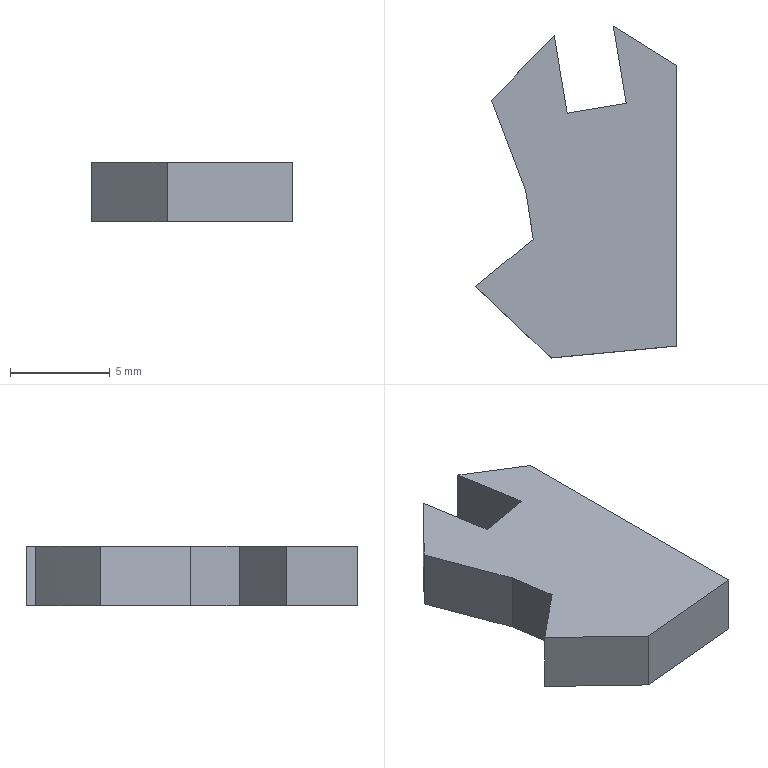Part | SolidWorks | features BaseBody 1 | 1 solid | 13 faces | box 10.052 x 16.622 x 3 mm | volume 347.373 mm3 | spline 7 | plane 6
STEP:
#1=CARTESIAN_POINT('',(-6.421,0.002241,-1.5));
#2=VERTEX_POINT('',#1);
#3=CARTESIAN_POINT('',(-0.1475,0.5984,-1.5));
#4=VERTEX_POINT('',#3);
#5=CARTESIAN_POINT('',(-6.421,0.002241,-1.5));
#6=CARTESIAN_POINT('',(-4.332,0.1996,-1.5));
#7=CARTESIAN_POINT('',(-0.1475,0.5984,-1.5));
#8=B_SPLINE_CURVE_WITH_KNOTS('',2,(#5,#6,#7),.UNSPECIFIED.,.F.,.F.,(3,3),(0.,0.05556),.UNSPECIFIED.);
#9=EDGE_CURVE('',#2,#4,#8,.T.);
#10=ORIENTED_EDGE('',*,*,#9,.F.);
#11=CARTESIAN_POINT('',(-10.2,3.587,-1.5));
#12=VERTEX_POINT('',#11);
#13=CARTESIAN_POINT('',(-10.2,3.587,-1.5));
#14=CARTESIAN_POINT('',(-8.939,2.393,-1.5));
#15=CARTESIAN_POINT('',(-7.681,1.198,-1.5));
#16=CARTESIAN_POINT('',(-6.421,0.002241,-1.5));
#17=B_SPLINE_CURVE_WITH_KNOTS('',3,(#13,#14,#15,#16),.UNSPECIFIED.,.F.,.F.,(4,4),(0.05556,0.1111),.UNSPECIFIED.);
#18=EDGE_CURVE('',#12,#2,#17,.T.);
#19=ORIENTED_EDGE('',*,*,#18,.F.);
#20=CARTESIAN_POINT('',(-7.315,5.947,-1.5));
#21=VERTEX_POINT('',#20);
#22=CARTESIAN_POINT('',(-7.315,5.947,-1.5));
#23=CARTESIAN_POINT('',(-8.275,5.16,-1.5));
#24=CARTESIAN_POINT('',(-9.238,4.374,-1.5));
#25=CARTESIAN_POINT('',(-10.2,3.587,-1.5));
#26=B_SPLINE_CURVE_WITH_KNOTS('',3,(#22,#23,#24,#25),.UNSPECIFIED.,.F.,.F.,(4,4),(0.1111,0.1667),.UNSPECIFIED.);
#27=EDGE_CURVE('',#21,#12,#26,.T.);
#28=ORIENTED_EDGE('',*,*,#27,.F.);
#29=CARTESIAN_POINT('',(-7.695,8.398,-1.5));
#30=VERTEX_POINT('',#29);
#31=CARTESIAN_POINT('',(-7.695,8.398,-1.5));
#32=CARTESIAN_POINT('',(-7.57,7.58,-1.5));
#33=CARTESIAN_POINT('',(-7.442,6.765,-1.5));
#34=CARTESIAN_POINT('',(-7.315,5.947,-1.5));
#35=B_SPLINE_CURVE_WITH_KNOTS('',3,(#31,#32,#33,#34),.UNSPECIFIED.,.F.,.F.,(4,4),(0.1667,0.2222),.UNSPECIFIED.);
#36=EDGE_CURVE('',#30,#21,#35,.T.);
#37=ORIENTED_EDGE('',*,*,#36,.F.);
#38=CARTESIAN_POINT('',(-9.403,12.915,-1.5));
#39=VERTEX_POINT('',#38);
#40=CARTESIAN_POINT('',(-9.403,12.915,-1.5));
#41=CARTESIAN_POINT('',(-8.834,11.41,-1.5));
#42=CARTESIAN_POINT('',(-8.265,9.904,-1.5));
#43=CARTESIAN_POINT('',(-7.695,8.398,-1.5));
#44=B_SPLINE_CURVE_WITH_KNOTS('',3,(#40,#41,#42,#43),.UNSPECIFIED.,.F.,.F.,(4,4),(0.2222,0.2778),.UNSPECIFIED.);
#45=EDGE_CURVE('',#39,#30,#44,.T.);
#46=ORIENTED_EDGE('',*,*,#45,.F.);
#47=CARTESIAN_POINT('',(-6.263,16.129,-1.5));
#48=VERTEX_POINT('',#47);
#49=CARTESIAN_POINT('',(-6.263,16.129,-1.5));
#50=CARTESIAN_POINT('',(-8.357,13.987,-1.5));
#51=CARTESIAN_POINT('',(-9.403,12.915,-1.5));
#52=B_SPLINE_CURVE_WITH_KNOTS('',2,(#49,#50,#51),.UNSPECIFIED.,.F.,.F.,(3,3),(0.2778,0.3333),.UNSPECIFIED.);
#53=EDGE_CURVE('',#48,#39,#52,.T.);
#54=ORIENTED_EDGE('',*,*,#53,.F.);
#55=CARTESIAN_POINT('',(-5.612,12.258,-1.5));
#56=VERTEX_POINT('',#55);
#57=CARTESIAN_POINT('',(-5.612,12.258,-1.5));
#58=DIRECTION('',(-0.1659,0.9861,0.));
#59=VECTOR('',#58,1000.);
#60=LINE('',#57,#59);
#61=EDGE_CURVE('',#56,#48,#60,.T.);
#62=ORIENTED_EDGE('',*,*,#61,.F.);
#63=CARTESIAN_POINT('',(-2.654,12.756,-1.5));
#64=VERTEX_POINT('',#63);
#65=CARTESIAN_POINT('',(-2.654,12.756,-1.5));
#66=DIRECTION('',(-0.9861,-0.1659,0.));
#67=VECTOR('',#66,1000.);
#68=LINE('',#65,#67);
#69=EDGE_CURVE('',#64,#56,#68,.T.);
#70=ORIENTED_EDGE('',*,*,#69,.F.);
#71=CARTESIAN_POINT('',(-3.305,16.624,-1.5));
#72=VERTEX_POINT('',#71);
#73=CARTESIAN_POINT('',(-2.654,12.756,-1.5));
#74=DIRECTION('',(0.1659,-0.9861,0.));
#75=VECTOR('',#74,1000.);
#76=LINE('',#73,#75);
#77=EDGE_CURVE('',#72,#64,#76,.T.);
#78=ORIENTED_EDGE('',*,*,#77,.F.);
#79=CARTESIAN_POINT('',(-0.1475,14.641,-1.5));
#80=VERTEX_POINT('',#79);
#81=CARTESIAN_POINT('',(-0.1475,14.641,-1.5));
#82=CARTESIAN_POINT('',(-1.178,15.289,-1.5));
#83=CARTESIAN_POINT('',(-3.21,16.565,-1.5));
#84=CARTESIAN_POINT('',(-3.305,16.624,-1.5));
#85=B_SPLINE_CURVE_WITH_KNOTS('',3,(#81,#82,#83,#84),.UNSPECIFIED.,.F.,.F.,(4,4),(0.8346,0.8889),.UNSPECIFIED.);
#86=EDGE_CURVE('',#80,#72,#85,.T.);
#87=ORIENTED_EDGE('',*,*,#86,.F.);
#88=CARTESIAN_POINT('',(-0.1475,14.641,-1.5));
#89=DIRECTION('',(0.,1.,0.));
#90=VECTOR('',#89,1000.);
#91=LINE('',#88,#90);
#92=EDGE_CURVE('',#4,#80,#91,.T.);
#93=ORIENTED_EDGE('',*,*,#92,.F.);
#94=EDGE_LOOP('',(#10,#19,#28,#37,#46,#54,#62,#70,#78,#87,#93));
#95=FACE_OUTER_BOUND('',#94,.T.);
#96=CARTESIAN_POINT('',(-3.808,0.25,-1.5));
#97=DIRECTION('',(0.,0.,1.));
#98=DIRECTION('',(1.,0.,0.));
#99=AXIS2_PLACEMENT_3D('',#96,#97,#98);
#100=PLANE('',#99);
#101=ADVANCED_FACE('',(#95),#100,.F.);
#102=CARTESIAN_POINT('',(-6.421,0.002241,1.5));
#103=VERTEX_POINT('',#102);
#104=CARTESIAN_POINT('',(-0.1475,0.5984,1.5));
#105=VERTEX_POINT('',#104);
#106=CARTESIAN_POINT('',(-6.421,0.002241,1.5));
#107=CARTESIAN_POINT('',(-4.332,0.1996,1.5));
#108=CARTESIAN_POINT('',(-0.1475,0.5984,1.5));
#109=B_SPLINE_CURVE_WITH_KNOTS('',2,(#106,#107,#108),.UNSPECIFIED.,.F.,.F.,(3,3),(0.,0.05556),.UNSPECIFIED.);
#110=EDGE_CURVE('',#103,#105,#109,.T.);
#111=ORIENTED_EDGE('',*,*,#110,.T.);
#112=CARTESIAN_POINT('',(-0.1475,14.641,1.5));
#113=VERTEX_POINT('',#112);
#114=CARTESIAN_POINT('',(-0.1475,14.641,1.5));
#115=DIRECTION('',(0.,1.,0.));
#116=VECTOR('',#115,1000.);
#117=LINE('',#114,#116);
#118=EDGE_CURVE('',#105,#113,#117,.T.);
#119=ORIENTED_EDGE('',*,*,#118,.T.);
#120=CARTESIAN_POINT('',(-3.305,16.624,1.5));
#121=VERTEX_POINT('',#120);
#122=CARTESIAN_POINT('',(-0.1475,14.641,1.5));
#123=CARTESIAN_POINT('',(-1.178,15.289,1.5));
#124=CARTESIAN_POINT('',(-3.21,16.565,1.5));
#125=CARTESIAN_POINT('',(-3.305,16.624,1.5));
#126=B_SPLINE_CURVE_WITH_KNOTS('',3,(#122,#123,#124,#125),.UNSPECIFIED.,.F.,.F.,(4,4),(0.8346,0.8889),.UNSPECIFIED.);
#127=EDGE_CURVE('',#113,#121,#126,.T.);
#128=ORIENTED_EDGE('',*,*,#127,.T.);
#129=CARTESIAN_POINT('',(-2.654,12.756,1.5));
#130=VERTEX_POINT('',#129);
#131=CARTESIAN_POINT('',(-2.654,12.756,1.5));
#132=DIRECTION('',(0.1659,-0.9861,0.));
#133=VECTOR('',#132,1000.);
#134=LINE('',#131,#133);
#135=EDGE_CURVE('',#121,#130,#134,.T.);
#136=ORIENTED_EDGE('',*,*,#135,.T.);
#137=CARTESIAN_POINT('',(-5.612,12.258,1.5));
#138=VERTEX_POINT('',#137);
#139=CARTESIAN_POINT('',(-2.654,12.756,1.5));
#140=DIRECTION('',(-0.9861,-0.1659,0.));
#141=VECTOR('',#140,1000.);
#142=LINE('',#139,#141);
#143=EDGE_CURVE('',#130,#138,#142,.T.);
#144=ORIENTED_EDGE('',*,*,#143,.T.);
#145=CARTESIAN_POINT('',(-6.263,16.129,1.5));
#146=VERTEX_POINT('',#145);
#147=CARTESIAN_POINT('',(-5.612,12.258,1.5));
#148=DIRECTION('',(-0.1659,0.9861,0.));
#149=VECTOR('',#148,1000.);
#150=LINE('',#147,#149);
#151=EDGE_CURVE('',#138,#146,#150,.T.);
#152=ORIENTED_EDGE('',*,*,#151,.T.);
#153=CARTESIAN_POINT('',(-9.403,12.915,1.5));
#154=VERTEX_POINT('',#153);
#155=CARTESIAN_POINT('',(-6.263,16.129,1.5));
#156=CARTESIAN_POINT('',(-8.357,13.987,1.5));
#157=CARTESIAN_POINT('',(-9.403,12.915,1.5));
#158=B_SPLINE_CURVE_WITH_KNOTS('',2,(#155,#156,#157),.UNSPECIFIED.,.F.,.F.,(3,3),(0.2778,0.3333),.UNSPECIFIED.);
#159=EDGE_CURVE('',#146,#154,#158,.T.);
#160=ORIENTED_EDGE('',*,*,#159,.T.);
#161=CARTESIAN_POINT('',(-7.695,8.398,1.5));
#162=VERTEX_POINT('',#161);
#163=CARTESIAN_POINT('',(-9.403,12.915,1.5));
#164=CARTESIAN_POINT('',(-8.834,11.41,1.5));
#165=CARTESIAN_POINT('',(-8.265,9.904,1.5));
#166=CARTESIAN_POINT('',(-7.695,8.398,1.5));
#167=B_SPLINE_CURVE_WITH_KNOTS('',3,(#163,#164,#165,#166),.UNSPECIFIED.,.F.,.F.,(4,4),(0.2222,0.2778),.UNSPECIFIED.);
#168=EDGE_CURVE('',#154,#162,#167,.T.);
#169=ORIENTED_EDGE('',*,*,#168,.T.);
#170=CARTESIAN_POINT('',(-7.315,5.947,1.5));
#171=VERTEX_POINT('',#170);
#172=CARTESIAN_POINT('',(-7.695,8.398,1.5));
#173=CARTESIAN_POINT('',(-7.57,7.58,1.5));
#174=CARTESIAN_POINT('',(-7.442,6.765,1.5));
#175=CARTESIAN_POINT('',(-7.315,5.947,1.5));
#176=B_SPLINE_CURVE_WITH_KNOTS('',3,(#172,#173,#174,#175),.UNSPECIFIED.,.F.,.F.,(4,4),(0.1667,0.2222),.UNSPECIFIED.);
#177=EDGE_CURVE('',#162,#171,#176,.T.);
#178=ORIENTED_EDGE('',*,*,#177,.T.);
#179=CARTESIAN_POINT('',(-10.2,3.587,1.5));
#180=VERTEX_POINT('',#179);
#181=CARTESIAN_POINT('',(-7.315,5.947,1.5));
#182=CARTESIAN_POINT('',(-8.275,5.16,1.5));
#183=CARTESIAN_POINT('',(-9.238,4.374,1.5));
#184=CARTESIAN_POINT('',(-10.2,3.587,1.5));
#185=B_SPLINE_CURVE_WITH_KNOTS('',3,(#181,#182,#183,#184),.UNSPECIFIED.,.F.,.F.,(4,4),(0.1111,0.1667),.UNSPECIFIED.);
#186=EDGE_CURVE('',#171,#180,#185,.T.);
#187=ORIENTED_EDGE('',*,*,#186,.T.);
#188=CARTESIAN_POINT('',(-10.2,3.587,1.5));
#189=CARTESIAN_POINT('',(-8.939,2.393,1.5));
#190=CARTESIAN_POINT('',(-7.681,1.198,1.5));
#191=CARTESIAN_POINT('',(-6.421,0.002241,1.5));
#192=B_SPLINE_CURVE_WITH_KNOTS('',3,(#188,#189,#190,#191),.UNSPECIFIED.,.F.,.F.,(4,4),(0.05556,0.1111),.UNSPECIFIED.);
#193=EDGE_CURVE('',#180,#103,#192,.T.);
#194=ORIENTED_EDGE('',*,*,#193,.T.);
#195=EDGE_LOOP('',(#111,#119,#128,#136,#144,#152,#160,#169,#178,#187,#194));
#196=FACE_OUTER_BOUND('',#195,.T.);
#197=CARTESIAN_POINT('',(-3.808,0.25,1.5));
#198=DIRECTION('',(0.,0.,1.));
#199=DIRECTION('',(1.,0.,0.));
#200=AXIS2_PLACEMENT_3D('',#197,#198,#199);
#201=PLANE('',#200);
#202=ADVANCED_FACE('',(#196),#201,.T.);
#203=ORIENTED_EDGE('',*,*,#18,.T.);
#204=CARTESIAN_POINT('',(-6.421,0.002241,1.5));
#205=DIRECTION('',(0.,0.,-1.));
#206=VECTOR('',#205,1000.);
#207=LINE('',#204,#206);
#208=EDGE_CURVE('',#103,#2,#207,.T.);
#209=ORIENTED_EDGE('',*,*,#208,.F.);
#210=ORIENTED_EDGE('',*,*,#193,.F.);
#211=CARTESIAN_POINT('',(-10.2,3.587,1.5));
#212=DIRECTION('',(0.,0.,-1.));
#213=VECTOR('',#212,1000.);
#214=LINE('',#211,#213);
#215=EDGE_CURVE('',#180,#12,#214,.T.);
#216=ORIENTED_EDGE('',*,*,#215,.T.);
#217=EDGE_LOOP('',(#203,#209,#210,#216));
#218=FACE_OUTER_BOUND('',#217,.T.);
#219=CARTESIAN_POINT('',(-10.2,3.587,1.5));
#220=CARTESIAN_POINT('',(-10.2,3.587,-1.5));
#221=CARTESIAN_POINT('',(-8.939,2.393,1.5));
#222=CARTESIAN_POINT('',(-8.939,2.393,-1.5));
#223=CARTESIAN_POINT('',(-7.681,1.198,1.5));
#224=CARTESIAN_POINT('',(-7.681,1.198,-1.5));
#225=CARTESIAN_POINT('',(-6.421,0.002241,1.5));
#226=CARTESIAN_POINT('',(-6.421,0.002241,-1.5));
#227=B_SPLINE_SURFACE_WITH_KNOTS('',3,1,((#219,#220),(#221,#222),(#223,#224),(#225,#226)),.UNSPECIFIED.,.F.,.F.,.F.,(4,4),(2,2),(0.05556,0.1111),(0.,1.),.UNSPECIFIED.);
#228=ADVANCED_FACE('',(#218),#227,.F.);
#229=ORIENTED_EDGE('',*,*,#27,.T.);
#230=ORIENTED_EDGE('',*,*,#215,.F.);
#231=ORIENTED_EDGE('',*,*,#186,.F.);
#232=CARTESIAN_POINT('',(-7.315,5.947,1.5));
#233=DIRECTION('',(0.,0.,-1.));
#234=VECTOR('',#233,1000.);
#235=LINE('',#232,#234);
#236=EDGE_CURVE('',#171,#21,#235,.T.);
#237=ORIENTED_EDGE('',*,*,#236,.T.);
#238=EDGE_LOOP('',(#229,#230,#231,#237));
#239=FACE_OUTER_BOUND('',#238,.T.);
#240=CARTESIAN_POINT('',(-7.315,5.947,1.5));
#241=CARTESIAN_POINT('',(-7.315,5.947,-1.5));
#242=CARTESIAN_POINT('',(-8.275,5.16,1.5));
#243=CARTESIAN_POINT('',(-8.275,5.16,-1.5));
#244=CARTESIAN_POINT('',(-9.238,4.374,1.5));
#245=CARTESIAN_POINT('',(-9.238,4.374,-1.5));
#246=CARTESIAN_POINT('',(-10.2,3.587,1.5));
#247=CARTESIAN_POINT('',(-10.2,3.587,-1.5));
#248=B_SPLINE_SURFACE_WITH_KNOTS('',3,1,((#240,#241),(#242,#243),(#244,#245),(#246,#247)),.UNSPECIFIED.,.F.,.F.,.F.,(4,4),(2,2),(0.1111,0.1667),(0.,1.),.UNSPECIFIED.);
#249=ADVANCED_FACE('',(#239),#248,.F.);
#250=ORIENTED_EDGE('',*,*,#36,.T.);
#251=ORIENTED_EDGE('',*,*,#236,.F.);
#252=ORIENTED_EDGE('',*,*,#177,.F.);
#253=CARTESIAN_POINT('',(-7.695,8.398,1.5));
#254=DIRECTION('',(0.,0.,-1.));
#255=VECTOR('',#254,1000.);
#256=LINE('',#253,#255);
#257=EDGE_CURVE('',#162,#30,#256,.T.);
#258=ORIENTED_EDGE('',*,*,#257,.T.);
#259=EDGE_LOOP('',(#250,#251,#252,#258));
#260=FACE_OUTER_BOUND('',#259,.T.);
#261=CARTESIAN_POINT('',(-7.695,8.398,1.5));
#262=CARTESIAN_POINT('',(-7.695,8.398,-1.5));
#263=CARTESIAN_POINT('',(-7.57,7.58,1.5));
#264=CARTESIAN_POINT('',(-7.57,7.58,-1.5));
#265=CARTESIAN_POINT('',(-7.442,6.765,1.5));
#266=CARTESIAN_POINT('',(-7.442,6.765,-1.5));
#267=CARTESIAN_POINT('',(-7.315,5.947,1.5));
#268=CARTESIAN_POINT('',(-7.315,5.947,-1.5));
#269=B_SPLINE_SURFACE_WITH_KNOTS('',3,1,((#261,#262),(#263,#264),(#265,#266),(#267,#268)),.UNSPECIFIED.,.F.,.F.,.F.,(4,4),(2,2),(0.1667,0.2222),(0.,1.),.UNSPECIFIED.);
#270=ADVANCED_FACE('',(#260),#269,.F.);
#271=ORIENTED_EDGE('',*,*,#45,.T.);
#272=ORIENTED_EDGE('',*,*,#257,.F.);
#273=ORIENTED_EDGE('',*,*,#168,.F.);
#274=CARTESIAN_POINT('',(-9.403,12.915,1.5));
#275=DIRECTION('',(0.,0.,-1.));
#276=VECTOR('',#275,1000.);
#277=LINE('',#274,#276);
#278=EDGE_CURVE('',#154,#39,#277,.T.);
#279=ORIENTED_EDGE('',*,*,#278,.T.);
#280=EDGE_LOOP('',(#271,#272,#273,#279));
#281=FACE_OUTER_BOUND('',#280,.T.);
#282=CARTESIAN_POINT('',(-9.403,12.915,1.5));
#283=CARTESIAN_POINT('',(-9.403,12.915,-1.5));
#284=CARTESIAN_POINT('',(-8.834,11.41,1.5));
#285=CARTESIAN_POINT('',(-8.834,11.41,-1.5));
#286=CARTESIAN_POINT('',(-8.265,9.904,1.5));
#287=CARTESIAN_POINT('',(-8.265,9.904,-1.5));
#288=CARTESIAN_POINT('',(-7.695,8.398,1.5));
#289=CARTESIAN_POINT('',(-7.695,8.398,-1.5));
#290=B_SPLINE_SURFACE_WITH_KNOTS('',3,1,((#282,#283),(#284,#285),(#286,#287),(#288,#289)),.UNSPECIFIED.,.F.,.F.,.F.,(4,4),(2,2),(0.2222,0.2778),(0.,1.),.UNSPECIFIED.);
#291=ADVANCED_FACE('',(#281),#290,.F.);
#292=ORIENTED_EDGE('',*,*,#53,.T.);
#293=ORIENTED_EDGE('',*,*,#278,.F.);
#294=ORIENTED_EDGE('',*,*,#159,.F.);
#295=CARTESIAN_POINT('',(-6.263,16.129,1.5));
#296=DIRECTION('',(0.,0.,-1.));
#297=VECTOR('',#296,1000.);
#298=LINE('',#295,#297);
#299=EDGE_CURVE('',#146,#48,#298,.T.);
#300=ORIENTED_EDGE('',*,*,#299,.T.);
#301=EDGE_LOOP('',(#292,#293,#294,#300));
#302=FACE_OUTER_BOUND('',#301,.T.);
#303=CARTESIAN_POINT('',(-6.263,16.129,1.5));
#304=CARTESIAN_POINT('',(-6.263,16.129,-1.5));
#305=CARTESIAN_POINT('',(-8.357,13.987,1.5));
#306=CARTESIAN_POINT('',(-8.357,13.987,-1.5));
#307=CARTESIAN_POINT('',(-9.403,12.915,1.5));
#308=CARTESIAN_POINT('',(-9.403,12.915,-1.5));
#309=B_SPLINE_SURFACE_WITH_KNOTS('',2,1,((#303,#304),(#305,#306),(#307,#308)),.UNSPECIFIED.,.F.,.F.,.F.,(3,3),(2,2),(0.2778,0.3333),(0.,1.),.UNSPECIFIED.);
#310=ADVANCED_FACE('',(#302),#309,.F.);
#311=ORIENTED_EDGE('',*,*,#61,.T.);
#312=ORIENTED_EDGE('',*,*,#299,.F.);
#313=ORIENTED_EDGE('',*,*,#151,.F.);
#314=CARTESIAN_POINT('',(-5.612,12.258,1.5));
#315=DIRECTION('',(0.,0.,-1.));
#316=VECTOR('',#315,1000.);
#317=LINE('',#314,#316);
#318=EDGE_CURVE('',#138,#56,#317,.T.);
#319=ORIENTED_EDGE('',*,*,#318,.T.);
#320=EDGE_LOOP('',(#311,#312,#313,#319));
#321=FACE_OUTER_BOUND('',#320,.T.);
#322=CARTESIAN_POINT('',(-5.612,12.258,1.5));
#323=DIRECTION('',(-0.9861,-0.1659,0.));
#324=DIRECTION('',(-0.1659,0.9861,0.));
#325=AXIS2_PLACEMENT_3D('',#322,#323,#324);
#326=PLANE('',#325);
#327=ADVANCED_FACE('',(#321),#326,.F.);
#328=ORIENTED_EDGE('',*,*,#69,.T.);
#329=ORIENTED_EDGE('',*,*,#318,.F.);
#330=ORIENTED_EDGE('',*,*,#143,.F.);
#331=CARTESIAN_POINT('',(-2.654,12.756,1.5));
#332=DIRECTION('',(0.,0.,-1.));
#333=VECTOR('',#332,1000.);
#334=LINE('',#331,#333);
#335=EDGE_CURVE('',#130,#64,#334,.T.);
#336=ORIENTED_EDGE('',*,*,#335,.T.);
#337=EDGE_LOOP('',(#328,#329,#330,#336));
#338=FACE_OUTER_BOUND('',#337,.T.);
#339=CARTESIAN_POINT('',(-2.654,12.756,1.5));
#340=DIRECTION('',(0.1659,-0.9861,0.));
#341=DIRECTION('',(0.,0.,-1.));
#342=AXIS2_PLACEMENT_3D('',#339,#340,#341);
#343=PLANE('',#342);
#344=ADVANCED_FACE('',(#338),#343,.F.);
#345=ORIENTED_EDGE('',*,*,#77,.T.);
#346=ORIENTED_EDGE('',*,*,#335,.F.);
#347=ORIENTED_EDGE('',*,*,#135,.F.);
#348=CARTESIAN_POINT('',(-3.305,16.624,1.5));
#349=DIRECTION('',(0.,0.,-1.));
#350=VECTOR('',#349,1000.);
#351=LINE('',#348,#350);
#352=EDGE_CURVE('',#121,#72,#351,.T.);
#353=ORIENTED_EDGE('',*,*,#352,.T.);
#354=EDGE_LOOP('',(#345,#346,#347,#353));
#355=FACE_OUTER_BOUND('',#354,.T.);
#356=CARTESIAN_POINT('',(-2.654,12.756,1.5));
#357=DIRECTION('',(0.9861,0.1659,0.));
#358=DIRECTION('',(0.,0.,-1.));
#359=AXIS2_PLACEMENT_3D('',#356,#357,#358);
#360=PLANE('',#359);
#361=ADVANCED_FACE('',(#355),#360,.F.);
#362=ORIENTED_EDGE('',*,*,#86,.T.);
#363=ORIENTED_EDGE('',*,*,#352,.F.);
#364=ORIENTED_EDGE('',*,*,#127,.F.);
#365=CARTESIAN_POINT('',(-0.1475,14.641,1.5));
#366=DIRECTION('',(0.,0.,-1.));
#367=VECTOR('',#366,1000.);
#368=LINE('',#365,#367);
#369=EDGE_CURVE('',#113,#80,#368,.T.);
#370=ORIENTED_EDGE('',*,*,#369,.T.);
#371=EDGE_LOOP('',(#362,#363,#364,#370));
#372=FACE_OUTER_BOUND('',#371,.T.);
#373=CARTESIAN_POINT('',(-0.1475,14.641,1.5));
#374=CARTESIAN_POINT('',(-0.1475,14.641,-1.5));
#375=CARTESIAN_POINT('',(-1.178,15.289,1.5));
#376=CARTESIAN_POINT('',(-1.178,15.289,-1.5));
#377=CARTESIAN_POINT('',(-3.21,16.565,1.5));
#378=CARTESIAN_POINT('',(-3.21,16.565,-1.5));
#379=CARTESIAN_POINT('',(-3.305,16.624,1.5));
#380=CARTESIAN_POINT('',(-3.305,16.624,-1.5));
#381=B_SPLINE_SURFACE_WITH_KNOTS('',3,1,((#373,#374),(#375,#376),(#377,#378),(#379,#380)),.UNSPECIFIED.,.F.,.F.,.F.,(4,4),(2,2),(0.8346,0.8889),(0.,1.),.UNSPECIFIED.);
#382=ADVANCED_FACE('',(#372),#381,.F.);
#383=ORIENTED_EDGE('',*,*,#92,.T.);
#384=ORIENTED_EDGE('',*,*,#369,.F.);
#385=ORIENTED_EDGE('',*,*,#118,.F.);
#386=CARTESIAN_POINT('',(-0.1475,0.5984,1.5));
#387=DIRECTION('',(0.,0.,-1.));
#388=VECTOR('',#387,1000.);
#389=LINE('',#386,#388);
#390=EDGE_CURVE('',#105,#4,#389,.T.);
#391=ORIENTED_EDGE('',*,*,#390,.T.);
#392=EDGE_LOOP('',(#383,#384,#385,#391));
#393=FACE_OUTER_BOUND('',#392,.T.);
#394=CARTESIAN_POINT('',(-0.1475,14.641,1.5));
#395=DIRECTION('',(-1.,0.,0.));
#396=DIRECTION('',(0.,0.,1.));
#397=AXIS2_PLACEMENT_3D('',#394,#395,#396);
#398=PLANE('',#397);
#399=ADVANCED_FACE('',(#393),#398,.F.);
#400=ORIENTED_EDGE('',*,*,#9,.T.);
#401=ORIENTED_EDGE('',*,*,#390,.F.);
#402=ORIENTED_EDGE('',*,*,#110,.F.);
#403=ORIENTED_EDGE('',*,*,#208,.T.);
#404=EDGE_LOOP('',(#400,#401,#402,#403));
#405=FACE_OUTER_BOUND('',#404,.T.);
#406=CARTESIAN_POINT('',(-6.421,0.002241,1.5));
#407=CARTESIAN_POINT('',(-6.421,0.002241,-1.5));
#408=CARTESIAN_POINT('',(-4.332,0.1996,1.5));
#409=CARTESIAN_POINT('',(-4.332,0.1996,-1.5));
#410=CARTESIAN_POINT('',(-0.1475,0.5984,1.5));
#411=CARTESIAN_POINT('',(-0.1475,0.5984,-1.5));
#412=B_SPLINE_SURFACE_WITH_KNOTS('',2,1,((#406,#407),(#408,#409),(#410,#411)),.UNSPECIFIED.,.F.,.F.,.F.,(3,3),(2,2),(0.,0.05556),(0.,1.),.UNSPECIFIED.);
#413=ADVANCED_FACE('',(#405),#412,.F.);
#414=CLOSED_SHELL('',(#101,#202,#228,#249,#270,#291,#310,#327,#344,#361,#382,#399,#413));
#415=MANIFOLD_SOLID_BREP('',#414);
#416=CARTESIAN_POINT('',(0.,0.,0.));
#417=DIRECTION('',(0.,0.,1.));
#418=DIRECTION('',(1.,0.,0.));
#419=AXIS2_PLACEMENT_3D('',#416,#417,#418);
#420=(LENGTH_UNIT()NAMED_UNIT(*)SI_UNIT(.MILLI.,.METRE.));
#421=UNCERTAINTY_MEASURE_WITH_UNIT(LENGTH_MEASURE(0.00001),#420,'','');
#422=(NAMED_UNIT(*)PLANE_ANGLE_UNIT()SI_UNIT($,.RADIAN.));
#423=(NAMED_UNIT(*)SI_UNIT($,.STERADIAN.)SOLID_ANGLE_UNIT());
#424=(GEOMETRIC_REPRESENTATION_CONTEXT(3)GLOBAL_UNCERTAINTY_ASSIGNED_CONTEXT((#421))GLOBAL_UNIT_ASSIGNED_CONTEXT((#420,#422,#423))REPRESENTATION_CONTEXT('',''));
#425=ADVANCED_BREP_SHAPE_REPRESENTATION('',(#415,#419),#424);